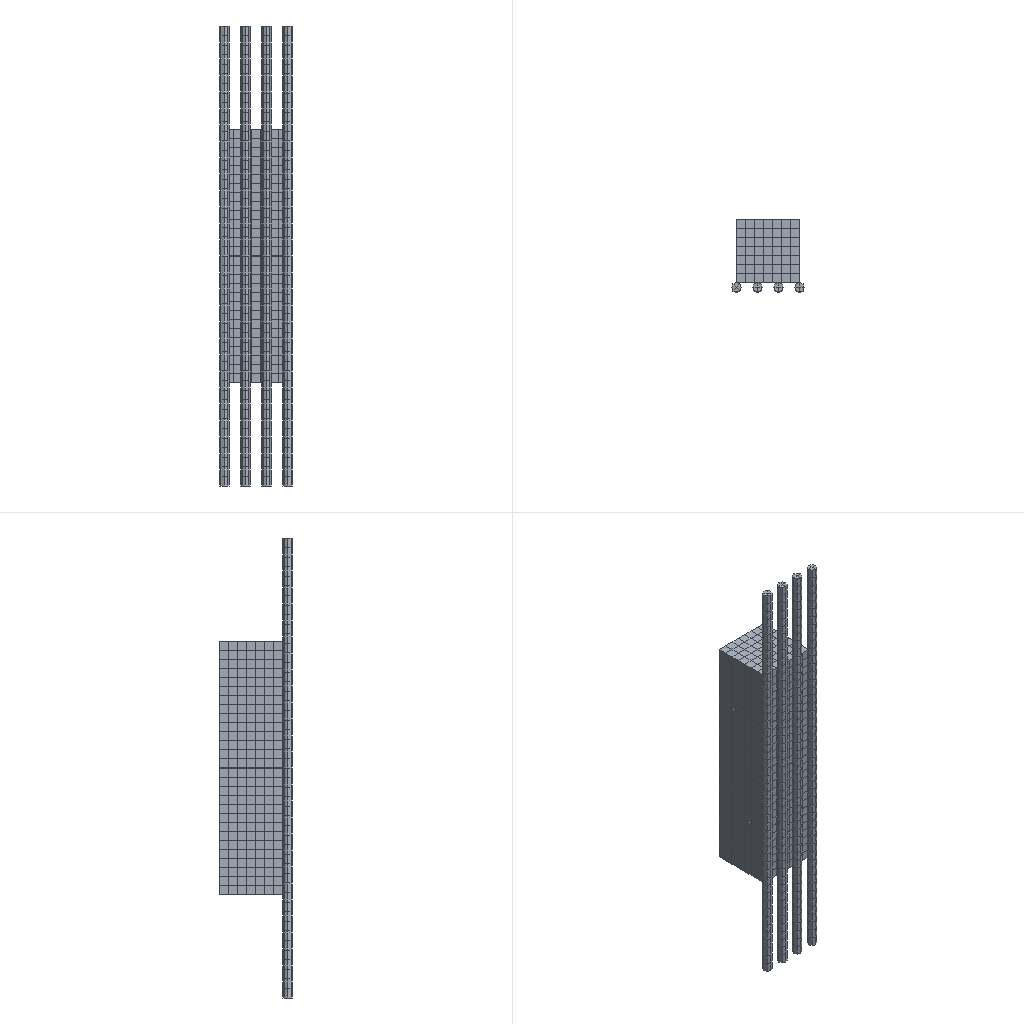Simulation study | abaqus
Set-up summary:
category,name,step,type,value,unit,region
solver,abaqus
solver,version,,,Abaqus/Standard 2020
units,not stated in the deck,,not stated
analysis,deck,,static,static
load_step,Step-G,Step-G,static
load_step,Step-1,Step-1,transient
load_step,requested,,,2
mesh,nodes,,,3812
mesh,elements,,,2140
element_type,C3D8R,,solid,2140
load,load commands in deck,,count,2
bc,support commands in deck,,count,12
material,GUNZI,,in results
material,MATERIAL-2,,in results
check,setup vs results,,match,"per instance, exact: element labels, types and connectivity; labels of the nodes the elements use; coordinates of those nodes at SINGLE_PRECISION in 8 of 8 instance(s)"
Abaqus input file, long lists of numbers shortened:
*Heading
** Job name: Job-1 Model name: Model-1
** Generated by: Abaqus/CAE 2020
*Preprint, echo=NO, model=NO, history=NO, contact=NO
**
** PARTS
**
*Part, name=work-1
*Node
      1,         330.,          25.,        331.5
      2,         330.,   72.143,        331.5
** (510 more lines like these left out)
*Element, type=C3D8R
  1,  65,  66,  74,  73,   1,   2,  10,   9
  2,  66,  67,  75,  74,   2,   3,  11,  10
** (341 more lines like these left out)
*Nset, nset=Set-1, generate
   1,  512,    1
*Elset, elset=Set-1, generate
   1,  343,    1
** Section: kuai
*Solid Section, elset=Set-1, material=Material-2
,
*End Part
**
*Part, name=work-2
*Node
      1,         330.,         355.,       -331.5
      2,         330.,   307.857,       -331.5
** (510 more lines like these left out)
*Element, type=C3D8R
  1,  65,  66,  74,  73,   1,   2,  10,   9
  2,  66,  67,  75,  74,   2,   3,  11,  10
** (341 more lines like these left out)
*Nset, nset=Set-1, generate
   1,  512,    1
*Elset, elset=Set-1, generate
   1,  343,    1
** Section: kuai
*Solid Section, elset=Set-1, material=Material-2
,
*End Part
**
*Part, name=work-3
*Node
      1,         330.,         355.,         -0.5
      2,         330.,   307.857,         -0.5
** (510 more lines like these left out)
*Element, type=C3D8R
  1,  65,  66,  74,  73,   1,   2,  10,   9
  2,  66,  67,  75,  74,   2,   3,  11,  10
** (341 more lines like these left out)
*Nset, nset=Set-1, generate
   1,  512,    1
*Elset, elset=Set-1, generate
   1,  343,    1
** Section: kuai
*Solid Section, elset=Set-1, material=Material-2
,
*End Part
**
*Part, name=work-4
*Node
      1,         330.,          25.,          0.5
      2,         330.,   72.143,          0.5
** (510 more lines like these left out)
*Element, type=C3D8R
  1,  65,  66,  74,  73,   1,   2,  10,   9
  2,  66,  67,  75,  74,   2,   3,  11,  10
** (341 more lines like these left out)
*Nset, nset=Set-1, generate
   1,  512,    1
*Elset, elset=Set-1, generate
   1,  343,    1
** Section: kuai
*Solid Section, elset=Set-1, material=Material-2
,
*End Part
**
*Part, name=work-71
*Node
      1,   312.322,  -17.678,      -1198.5
      2,         330.,         -25.,      -1198.5
** (439 more lines like these left out)
*Element, type=C3D8R
  1,   4,   1,   2,   9,  13,  10,  11,  18
  2,   2,   3,   5,   9,  11,  12,  14,  18
** (190 more lines like these left out)
*Nset, nset=Set-1, generate
   1,  441,    1
*Elset, elset=Set-1, generate
   1,  192,    1
** Section: sic
*Solid Section, elset=Set-1, material=GUNZI
,
*End Part
**
*Part, name=work-72
*Node
      1,   202.322,  -17.678,      -1198.5
      2,         220.,         -25.,      -1198.5
** (439 more lines like these left out)
*Element, type=C3D8R
  1,   4,   1,   2,   9,  13,  10,  11,  18
  2,   4,   9,   7,   8,  13,  18,  16,  17
** (190 more lines like these left out)
*Nset, nset=Set-1, generate
   1,  441,    1
*Elset, elset=Set-1, generate
   1,  192,    1
** Section: sic
*Solid Section, elset=Set-1, material=GUNZI
,
*End Part
**
*Part, name=work-73
*Node
      1,   92.322,  -17.678,      -1198.5
      2,         110.,         -25.,      -1198.5
** (439 more lines like these left out)
*Element, type=C3D8R
  1,   4,   1,   2,   9,  13,  10,  11,  18
  2,   5,   9,   2,   3,  14,  18,  11,  12
** (190 more lines like these left out)
*Nset, nset=Set-1, generate
   1,  441,    1
*Elset, elset=Set-1, generate
   1,  192,    1
** Section: sic
*Solid Section, elset=Set-1, material=GUNZI
,
*End Part
**
*Part, name=work-75
*Node
      1,  -17.678,  -17.678,      -1198.5
      2,           0.,         -25.,      -1198.5
** (439 more lines like these left out)
*Element, type=C3D8R
  1,   3,   9,   1,   2,  12,  18,  10,  11
  2,   8,   4,   1,   9,  17,  13,  10,  18
** (190 more lines like these left out)
*Nset, nset=Set-1, generate
   1,  441,    1
*Elset, elset=Set-1, generate
   1,  192,    1
** Section: sic
*Solid Section, elset=Set-1, material=GUNZI
,
*End Part
**
**
** ASSEMBLY
**
*Assembly, name=Assembly
**
*Instance, name=work-1-1, part=work-1
*End Instance
**
*Instance, name=work-2-1, part=work-2
*End Instance
**
*Instance, name=work-3-1, part=work-3
*End Instance
**
*Instance, name=work-4-1, part=work-4
*End Instance
**
*Instance, name=work-71-1, part=work-71
*End Instance
**
*Instance, name=work-72-1, part=work-72
*End Instance
**
*Instance, name=work-73-1, part=work-73
*End Instance
**
*Instance, name=work-75-1, part=work-75
*End Instance
**
*Node
      1, -1.77635684e-15, 5.70367634e-15,           0.
*Node
      2,         110., -3.63996061e-15,           0.
*Node
      3,         220., 5.70367634e-15,           0.
*Node
      4,         330., -2.36062119e-14,           0.
*Nset, nset=Set-1, instance=work-71-1
   1,   2,   3,   4,   5,   6,   7,   8,   9, 433, 434, 435, 436, 437, 438, 439
 440, 441
*Nset, nset=Set-1, instance=work-72-1
   1,   2,   3,   4,   5,   6,   7,   8,   9, 433, 434, 435, 436, 437, 438, 439
 440, 441
*Nset, nset=Set-1, instance=work-73-1
   1,   2,   3,   4,   5,   6,   7,   8,   9, 433, 434, 435, 436, 437, 438, 439
 440, 441
*Nset, nset=Set-1, instance=work-75-1
   1,   2,   3,   4,   5,   6,   7,   8,   9, 433, 434, 435, 436, 437, 438, 439
 440, 441
*Elset, elset=Set-1, instance=work-71-1
   1,   2,   3,   4, 189, 190, 191, 192
*Elset, elset=Set-1, instance=work-72-1
   1,   2,   3,   4, 189, 190, 191, 192
*Elset, elset=Set-1, instance=work-73-1
   1,   2,   3,   4, 189, 190, 191, 192
*Elset, elset=Set-1, instance=work-75-1
   1,   2,   3,   4, 189, 190, 191, 192
*Nset, nset=Set-2, instance=work-1-1, generate
   1,  512,    1
*Nset, nset=Set-2, instance=work-2-1, generate
   1,  512,    1
*Nset, nset=Set-2, instance=work-4-1, generate
   1,  512,    1
*Nset, nset=Set-2, instance=work-3-1, generate
   1,  512,    1
*Elset, elset=Set-2, instance=work-1-1, generate
   1,  343,    1
*Elset, elset=Set-2, instance=work-2-1, generate
   1,  343,    1
*Elset, elset=Set-2, instance=work-4-1, generate
   1,  343,    1
*Elset, elset=Set-2, instance=work-3-1, generate
   1,  343,    1
*Nset, nset=Set-3, instance=work-71-1
   1,   2,   3,   4,   5,   6,   7,   8,   9, 433, 434, 435, 436, 437, 438, 439
 440, 441
*Nset, nset=Set-3, instance=work-72-1
   1,   2,   3,   4,   5,   6,   7,   8,   9, 433, 434, 435, 436, 437, 438, 439
 440, 441
*Nset, nset=Set-3, instance=work-73-1
   1,   2,   3,   4,   5,   6,   7,   8,   9, 433, 434, 435, 436, 437, 438, 439
 440, 441
*Nset, nset=Set-3, instance=work-75-1
   1,   2,   3,   4,   5,   6,   7,   8,   9, 433, 434, 435, 436, 437, 438, 439
 440, 441
*Elset, elset=Set-3, instance=work-71-1
   1,   2,   3,   4, 189, 190, 191, 192
*Elset, elset=Set-3, instance=work-72-1
   1,   2,   3,   4, 189, 190, 191, 192
*Elset, elset=Set-3, instance=work-73-1
   1,   2,   3,   4, 189, 190, 191, 192
*Elset, elset=Set-3, instance=work-75-1
   1,   2,   3,   4, 189, 190, 191, 192
*Nset, nset=Set-4, instance=work-71-1
   1,   2,   3,   4,   5,   6,   7,   8,   9, 433, 434, 435, 436, 437, 438, 439
 440, 441
*Nset, nset=Set-4, instance=work-72-1
   1,   2,   3,   4,   5,   6,   7,   8,   9, 433, 434, 435, 436, 437, 438, 439
 440, 441
*Nset, nset=Set-4, instance=work-73-1
   1,   2,   3,   4,   5,   6,   7,   8,   9, 433, 434, 435, 436, 437, 438, 439
 440, 441
*Nset, nset=Set-4, instance=work-75-1
   1,   2,   3,   4,   5,   6,   7,   8,   9, 433, 434, 435, 436, 437, 438, 439
 440, 441
*Elset, elset=Set-4, instance=work-71-1
   1,   2,   3,   4, 189, 190, 191, 192
*Elset, elset=Set-4, instance=work-72-1
   1,   2,   3,   4, 189, 190, 191, 192
*Elset, elset=Set-4, instance=work-73-1
   1,   2,   3,   4, 189, 190, 191, 192
*Elset, elset=Set-4, instance=work-75-1
   1,   2,   3,   4, 189, 190, 191, 192
*Nset, nset=Set-9, generate
 1,  4,  1
*Nset, nset=m_Set-5
 1,
*Nset, nset=m_Set-6
 2,
*Nset, nset=m_Set-7
 3,
*Nset, nset=m_Set-8
 4,
*Elset, elset=_m_Surf-1_S6, internal, instance=work-1-1, generate
   1,  337,    7
*Elset, elset=_m_Surf-1_S6, internal, instance=work-4-1, generate
   1,  337,    7
*Elset, elset=_m_Surf-1_S4, internal, instance=work-2-1, generate
   7,  343,    7
*Elset, elset=_m_Surf-1_S4, internal, instance=work-3-1, generate
   7,  343,    7
*Surface, type=ELEMENT, name=m_Surf-1
_m_Surf-1_S6, S6
_m_Surf-1_S4, S4
*Elset, elset=_m_Surf-3_S3, internal, instance=work-1-1
   1,   2,   3,   4,   5,   6,   7,  50,  51,  52,  53,  54,  55,  56,  99, 100
 101, 102, 103, 104, 105, 148, 149, 150, 151, 152, 153, 154, 197, 198, 199, 200
** (2 more lines like these left out)
*Surface, type=ELEMENT, name=m_Surf-3
_m_Surf-3_S3, S3
*Elset, elset=_m_Surf-5_S3, internal, instance=work-4-1
   1,   2,   3,   4,   5,   6,   7,  50,  51,  52,  53,  54,  55,  56,  99, 100
 101, 102, 103, 104, 105, 148, 149, 150, 151, 152, 153, 154, 197, 198, 199, 200
** (2 more lines like these left out)
*Surface, type=ELEMENT, name=m_Surf-5
_m_Surf-5_S3, S3
*Elset, elset=_m_Surf-7_S5, internal, instance=work-3-1
  43,  44,  45,  46,  47,  48,  49,  92,  93,  94,  95,  96,  97,  98, 141, 142
 143, 144, 145, 146, 147, 190, 191, 192, 193, 194, 195, 196, 239, 240, 241, 242
** (2 more lines like these left out)
*Surface, type=ELEMENT, name=m_Surf-7
_m_Surf-7_S5, S5
*Elset, elset=_s_Surf-1_S3, internal, instance=work-71-1
   1,   2,   5,   6,   9,  10,  13,  14,  17,  18,  21,  22,  25,  26,  29,  30
  33,  34,  37,  38,  41,  42,  45,  46,  49,  50,  53,  54,  57,  58,  61,  62
** (4 more lines like these left out)
*Elset, elset=_s_Surf-1_S3, internal, instance=work-72-1, generate
   1,  191,    2
*Elset, elset=_s_Surf-1_S3, internal, instance=work-73-1, generate
   1,  189,    4
*Elset, elset=_s_Surf-1_S3, internal, instance=work-75-1
   2,   3,   6,   7,  10,  11,  14,  15,  18,  19,  22,  23,  26,  27,  30,  31
  34,  35,  38,  39,  42,  43,  46,  47,  50,  51,  54,  55,  58,  59,  62,  63
** (4 more lines like these left out)
*Elset, elset=_s_Surf-1_S4, internal, instance=work-71-1
   1,   2,   5,   6,   9,  10,  13,  14,  17,  18,  21,  22,  25,  26,  29,  30
  33,  34,  37,  38,  41,  42,  45,  46,  49,  50,  53,  54,  57,  58,  61,  62
** (4 more lines like these left out)
*Elset, elset=_s_Surf-1_S4, internal, instance=work-72-1, generate
   1,  191,    2
*Elset, elset=_s_Surf-1_S4, internal, instance=work-73-1, generate
   1,  189,    4
*Elset, elset=_s_Surf-1_S4, internal, instance=work-75-1
   2,   3,   6,   7,  10,  11,  14,  15,  18,  19,  22,  23,  26,  27,  30,  31
  34,  35,  38,  39,  42,  43,  46,  47,  50,  51,  54,  55,  58,  59,  62,  63
** (4 more lines like these left out)
*Elset, elset=_s_Surf-1_S5, internal, instance=work-71-1
   3,   4,   7,   8,  11,  12,  15,  16,  19,  20,  23,  24,  27,  28,  31,  32
  35,  36,  39,  40,  43,  44,  47,  48,  51,  52,  55,  56,  59,  60,  63,  64
** (4 more lines like these left out)
*Elset, elset=_s_Surf-1_S5, internal, instance=work-72-1, generate
   2,  192,    2
*Elset, elset=_s_Surf-1_S5, internal, instance=work-73-1
   2,   3,   4,   6,   7,   8,  10,  11,  12,  14,  15,  16,  18,  19,  20,  22
  23,  24,  26,  27,  28,  30,  31,  32,  34,  35,  36,  38,  39,  40,  42,  43
** (7 more lines like these left out)
*Elset, elset=_s_Surf-1_S5, internal, instance=work-75-1
   1,   4,   5,   8,   9,  12,  13,  16,  17,  20,  21,  24,  25,  28,  29,  32
  33,  36,  37,  40,  41,  44,  45,  48,  49,  52,  53,  56,  57,  60,  61,  64
** (4 more lines like these left out)
*Elset, elset=_s_Surf-1_S6, internal, instance=work-71-1
   3,   4,   7,   8,  11,  12,  15,  16,  19,  20,  23,  24,  27,  28,  31,  32
  35,  36,  39,  40,  43,  44,  47,  48,  51,  52,  55,  56,  59,  60,  63,  64
** (4 more lines like these left out)
*Elset, elset=_s_Surf-1_S6, internal, instance=work-72-1, generate
   2,  192,    2
*Elset, elset=_s_Surf-1_S6, internal, instance=work-73-1
   2,   3,   4,   6,   7,   8,  10,  11,  12,  14,  15,  16,  18,  19,  20,  22
  23,  24,  26,  27,  28,  30,  31,  32,  34,  35,  36,  38,  39,  40,  42,  43
** (7 more lines like these left out)
*Elset, elset=_s_Surf-1_S6, internal, instance=work-75-1
   1,   4,   5,   8,   9,  12,  13,  16,  17,  20,  21,  24,  25,  28,  29,  32
  33,  36,  37,  40,  41,  44,  45,  48,  49,  52,  53,  56,  57,  60,  61,  64
** (4 more lines like these left out)
*Surface, type=ELEMENT, name=s_Surf-1
_s_Surf-1_S3, S3
_s_Surf-1_S4, S4
_s_Surf-1_S6, S6
_s_Surf-1_S5, S5
*Elset, elset=_s_Surf-3_S5, internal, instance=work-4-1
  43,  44,  45,  46,  47,  48,  49,  92,  93,  94,  95,  96,  97,  98, 141, 142
 143, 144, 145, 146, 147, 190, 191, 192, 193, 194, 195, 196, 239, 240, 241, 242
** (2 more lines like these left out)
*Surface, type=ELEMENT, name=s_Surf-3
_s_Surf-3_S5, S5
*Elset, elset=_s_Surf-5_S3, internal, instance=work-3-1
   1,   2,   3,   4,   5,   6,   7,  50,  51,  52,  53,  54,  55,  56,  99, 100
 101, 102, 103, 104, 105, 148, 149, 150, 151, 152, 153, 154, 197, 198, 199, 200
** (2 more lines like these left out)
*Surface, type=ELEMENT, name=s_Surf-5
_s_Surf-5_S3, S3
*Elset, elset=_s_Surf-7_S3, internal, instance=work-2-1
   1,   2,   3,   4,   5,   6,   7,  50,  51,  52,  53,  54,  55,  56,  99, 100
 101, 102, 103, 104, 105, 148, 149, 150, 151, 152, 153, 154, 197, 198, 199, 200
** (2 more lines like these left out)
*Surface, type=ELEMENT, name=s_Surf-7
_s_Surf-7_S3, S3
*Elset, elset=_s_Surf-9_S3, internal, instance=work-71-1
   1,   2,   5,   6,   9,  10,  13,  14,  17,  18,  21,  22,  25,  26,  29,  30
  33,  34,  37,  38,  41,  42,  45,  46,  49,  50,  53,  54,  57,  58,  61,  62
** (4 more lines like these left out)
*Elset, elset=_s_Surf-9_S3, internal, instance=work-72-1, generate
   1,  191,    2
*Elset, elset=_s_Surf-9_S3, internal, instance=work-73-1, generate
   1,  189,    4
*Elset, elset=_s_Surf-9_S3, internal, instance=work-75-1
   2,   3,   6,   7,  10,  11,  14,  15,  18,  19,  22,  23,  26,  27,  30,  31
  34,  35,  38,  39,  42,  43,  46,  47,  50,  51,  54,  55,  58,  59,  62,  63
** (4 more lines like these left out)
*Elset, elset=_s_Surf-9_S4, internal, instance=work-71-1
   1,   2,   5,   6,   9,  10,  13,  14,  17,  18,  21,  22,  25,  26,  29,  30
  33,  34,  37,  38,  41,  42,  45,  46,  49,  50,  53,  54,  57,  58,  61,  62
** (4 more lines like these left out)
*Elset, elset=_s_Surf-9_S4, internal, instance=work-72-1, generate
   1,  191,    2
*Elset, elset=_s_Surf-9_S4, internal, instance=work-73-1, generate
   1,  189,    4
*Elset, elset=_s_Surf-9_S4, internal, instance=work-75-1
   2,   3,   6,   7,  10,  11,  14,  15,  18,  19,  22,  23,  26,  27,  30,  31
  34,  35,  38,  39,  42,  43,  46,  47,  50,  51,  54,  55,  58,  59,  62,  63
** (4 more lines like these left out)
*Elset, elset=_s_Surf-9_S5, internal, instance=work-71-1
   3,   4,   7,   8,  11,  12,  15,  16,  19,  20,  23,  24,  27,  28,  31,  32
  35,  36,  39,  40,  43,  44,  47,  48,  51,  52,  55,  56,  59,  60,  63,  64
** (4 more lines like these left out)
*Elset, elset=_s_Surf-9_S5, internal, instance=work-72-1, generate
   2,  192,    2
*Elset, elset=_s_Surf-9_S5, internal, instance=work-73-1
   2,   3,   4,   6,   7,   8,  10,  11,  12,  14,  15,  16,  18,  19,  20,  22
  23,  24,  26,  27,  28,  30,  31,  32,  34,  35,  36,  38,  39,  40,  42,  43
** (7 more lines like these left out)
*Elset, elset=_s_Surf-9_S5, internal, instance=work-75-1
   1,   4,   5,   8,   9,  12,  13,  16,  17,  20,  21,  24,  25,  28,  29,  32
  33,  36,  37,  40,  41,  44,  45,  48,  49,  52,  53,  56,  57,  60,  61,  64
** (4 more lines like these left out)
*Elset, elset=_s_Surf-9_S6, internal, instance=work-71-1
   3,   4,   7,   8,  11,  12,  15,  16,  19,  20,  23,  24,  27,  28,  31,  32
  35,  36,  39,  40,  43,  44,  47,  48,  51,  52,  55,  56,  59,  60,  63,  64
** (4 more lines like these left out)
*Elset, elset=_s_Surf-9_S6, internal, instance=work-72-1, generate
   2,  192,    2
*Elset, elset=_s_Surf-9_S6, internal, instance=work-73-1
   2,   3,   4,   6,   7,   8,  10,  11,  12,  14,  15,  16,  18,  19,  20,  22
  23,  24,  26,  27,  28,  30,  31,  32,  34,  35,  36,  38,  39,  40,  42,  43
** (7 more lines like these left out)
*Elset, elset=_s_Surf-9_S6, internal, instance=work-75-1
   1,   4,   5,   8,   9,  12,  13,  16,  17,  20,  21,  24,  25,  28,  29,  32
  33,  36,  37,  40,  41,  44,  45,  48,  49,  52,  53,  56,  57,  60,  61,  64
** (4 more lines like these left out)
*Surface, type=ELEMENT, name=s_Surf-9
_s_Surf-9_S3, S3
_s_Surf-9_S4, S4
_s_Surf-9_S6, S6
_s_Surf-9_S5, S5
*Elset, elset=_s_Surf-10_S2, internal, instance=work-75-1, generate
 189,  192,    1
*Elset, elset=_s_Surf-10_S1, internal, instance=work-75-1, generate
 1,  4,  1
*Surface, type=ELEMENT, name=s_Surf-10
_s_Surf-10_S2, S2
_s_Surf-10_S1, S1
*Elset, elset=_s_Surf-11_S2, internal, instance=work-73-1, generate
 189,  192,    1
*Elset, elset=_s_Surf-11_S1, internal, instance=work-73-1, generate
 1,  4,  1
*Surface, type=ELEMENT, name=s_Surf-11
_s_Surf-11_S2, S2
_s_Surf-11_S1, S1
*Elset, elset=_s_Surf-12_S2, internal, instance=work-72-1, generate
 189,  192,    1
*Elset, elset=_s_Surf-12_S1, internal, instance=work-72-1, generate
 1,  4,  1
*Surface, type=ELEMENT, name=s_Surf-12
_s_Surf-12_S2, S2
_s_Surf-12_S1, S1
*Elset, elset=_s_Surf-13_S2, internal, instance=work-71-1, generate
 189,  192,    1
*Elset, elset=_s_Surf-13_S1, internal, instance=work-71-1, generate
 1,  4,  1
*Surface, type=ELEMENT, name=s_Surf-13
_s_Surf-13_S2, S2
_s_Surf-13_S1, S1
** Constraint: Constraint-1
*Coupling, constraint name=Constraint-1, ref node=m_Set-5, surface=s_Surf-10
*Kinematic
** Constraint: Constraint-2
*Coupling, constraint name=Constraint-2, ref node=m_Set-6, surface=s_Surf-11
*Kinematic
** Constraint: Constraint-3
*Coupling, constraint name=Constraint-3, ref node=m_Set-7, surface=s_Surf-12
*Kinematic
** Constraint: Constraint-4
*Coupling, constraint name=Constraint-4, ref node=m_Set-8, surface=s_Surf-13
*Kinematic
*End Assembly
*Amplitude, name=Amp-1
             0.,              0.,             10.,              1.
**
** MATERIALS
**
*Material, name=GUNZI
*Conductivity
36.,
*Density
 3.22e-09,
*Elastic
192000., 0.142
*Expansion
 4e-06,
*Specific Heat
 4.2e+08,
*Material, name=Material-2
*Density
 1.113e-09,
*Elastic
72000., 0.32
**
** INTERACTION PROPERTIES
**
*Surface Interaction, name=IntProp-1
1.,
*Friction, slip tolerance=0.005
 0.6,
*Surface Behavior, pressure-overclosure=HARD
*Gap Conductance
 0.5,   0.
  0., 0.01
*Surface Interaction, name=jiechu
1.,
*Friction, slip tolerance=0.005
 0.2,
*Surface Behavior, pressure-overclosure=HARD
**
** INTERACTIONS
**
** Interaction: Int-2
*Contact Pair, interaction=IntProp-1, small sliding
s_Surf-9, m_Surf-1
** Interaction: Int-3
*Contact Pair, interaction=jiechu, type=SURFACE TO SURFACE
s_Surf-3, m_Surf-3
** Interaction: Int-3-Copy
*Contact Pair, interaction=jiechu, type=SURFACE TO SURFACE
s_Surf-5, m_Surf-5
** Interaction: Int-3-Copy2
*Contact Pair, interaction=jiechu, type=SURFACE TO SURFACE
s_Surf-7, m_Surf-7
** ----------------------------------------------------------------
**
** STEP: Step-G
**
*Step, name=Step-G, nlgeom=YES, inc=1000
*Static, stabilize=0.0002, allsdtol=0.05, continue=NO
0.01, 1., 1e-05, 1.
**
** BOUNDARY CONDITIONS
**
** Name: BC-2 Type: 位移/转角
*Boundary
Set-9, 1, 1
Set-9, 2, 2
Set-9, 3, 3
Set-9, 4, 4
Set-9, 5, 5
Set-9, 6, 6
**
** LOADS
**
** Name: Load-1   Type: Gravity
*Dload
Set-2, GRAV, 9800., 0., -1., 0.
**
** OUTPUT REQUESTS
**
*Restart, write, frequency=0
**
** FIELD OUTPUT: F-Output-2
**
*Output, field
*Node Output
CF, NT, RF, RM, RT, U, V
*Element Output, directions=YES
E, LE, MISES, MISESMAX, PE, PEEQ, PEMAG, S, TEMP
*Contact Output
CDISP, CSTRESS
*Output, history, frequency=0
*End Step
** ----------------------------------------------------------------
**
** STEP: Step-1
**
*Step, name=Step-1, nlgeom=YES, inc=10000
*Dynamic
0.01,10.,1e-05
**
** BOUNDARY CONDITIONS
**
** Name: BC-2 Type: 位移/转角
*Boundary, amplitude=Amp-1
Set-9, 1, 1
Set-9, 2, 2
Set-9, 3, 3
Set-9, 4, 4
Set-9, 5, 5
Set-9, 6, 6, 6.281
**
** OUTPUT REQUESTS
**
*Restart, write, number interval=1, time marks=NO
**
** FIELD OUTPUT: F-Output-1
**
*Output, field, frequency=1
*Node Output
CF, NT, RF, RM, RT, U, V
*Element Output, directions=YES
E, LE, MISES, MISESMAX, PE, PEEQ, PEMAG, S, TEMP
*Contact Output
CDISP, CSTRESS
**
** FIELD OUTPUT: F-Output-2
**
*Output, field, frequency=1
*Node Output
CF, NT, RF, RM, RT, U, V
*Element Output, directions=YES
E, LE, MISES, MISESMAX, PE, PEEQ, PEMAG, S, TEMP
*Contact Output
CDISP, CSTRESS
**
** HISTORY OUTPUT: H-Output-1
**
*Output, history, variable=PRESELECT, number interval=200, time marks=NO
*End Step
Results summary:
result,step,,completed,increments=11 time=1.0/1.0
result,step,,partial,increments=178 time=6.639/10.0
result,analysis,,,transient
result,last_loadstep,,,2
result,primary field,,,U
result,reaction total,,FX,42.451,model units
result,reaction total,,FY,1483.006,model units
result,reaction total,,FZ,-43.294,model units